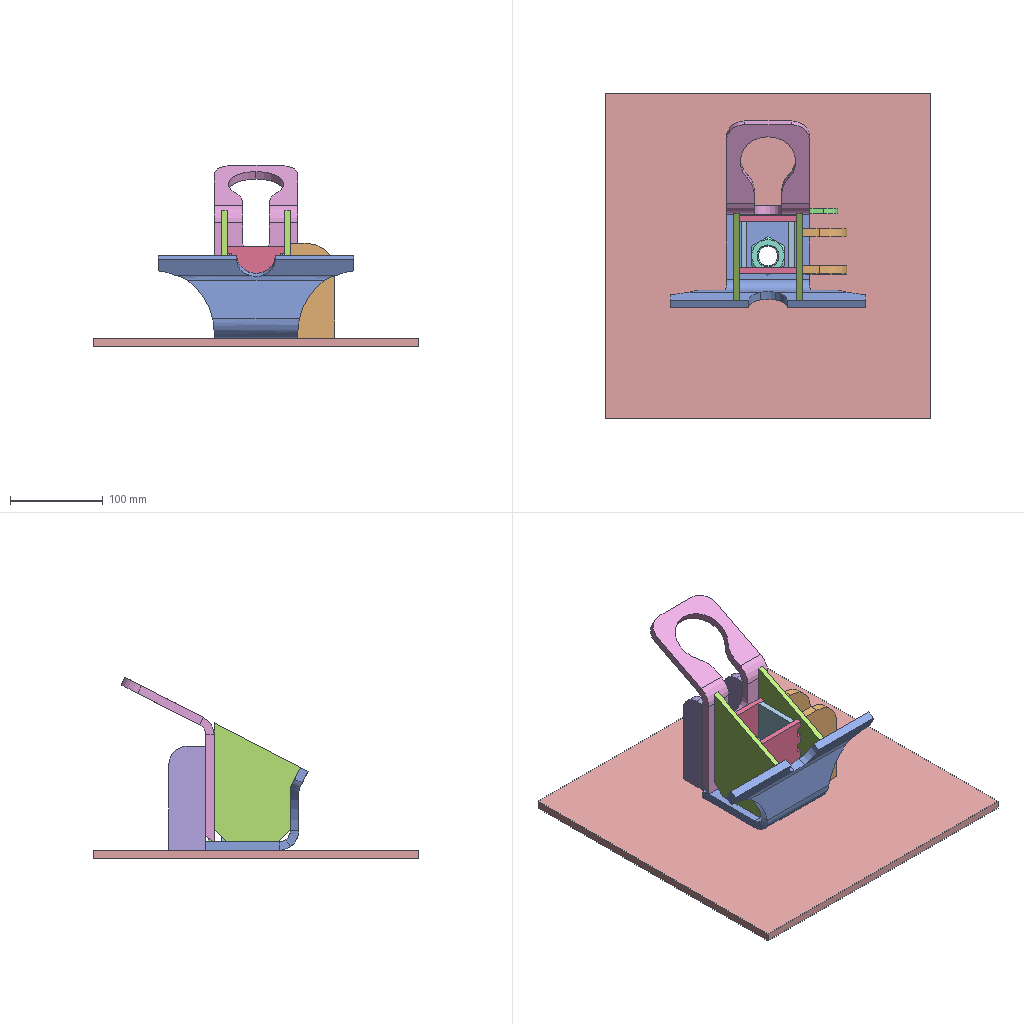Assembly | SolidWorks | 12 different items | 17 placed | box 350 x 350 x 195 mm
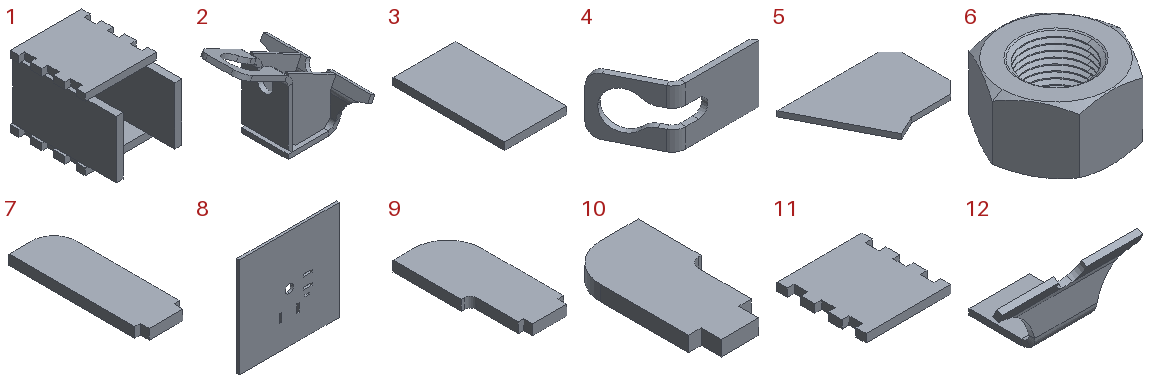Parts list (item | name | quantity | parent item | size | volume | features):
1 | (subassembly) | x1 | - | 62 x 90 x 62 mm | 98760 mm3 | -
2 | (subassembly) | x1 | - | 201.093 x 210 x 186 mm | 418946 mm3 | features CompositeCurve 1, MirrorCompFeat 1, ReferencePattern 1
3 | - | x2 | in 1 | 50 x 90 x 6 mm | 27000 mm3 | features FlatPattern 1, SMBaseFlange 1, SheetMetal 1
4 | - | x1 | in 2 | 177 x 100.092 x 90 mm | 136681 mm3 | features Fillet 2, Fold 2, ICE 2, UnFold 2, FlatPattern 1, SMBaseFlange 1, SheetMetal 1
5 | - | x2 | in 2 | 128 x 93 x 6 mm | 52464 mm3 | features FlatPattern 1, SMBaseFlange 1, SheetMetal 1
6 | - | x1 | in 2 | 41.569 x 36 x 21.5 mm | 15808 mm3 | features RevCut 2, Chamfer 1, Extrusion 1, LPattern 1
7 | - | x2 | - | 40 x 120 x 9 mm | 41707 mm3 | features FlatPattern 1, SMBaseFlange 1, SheetMetal 1
8 | - | x1 | - | 350 x 9 x 350 mm | 1086025 mm3 | features FlatPattern 1, ICE 1, SMBaseFlange 1, SheetMetal 1
9 | - | x2 | - | 48 x 110 x 9 mm | 41510 mm3 | features Fillet 1, FlatPattern 1, SMBaseFlange 1, SheetMetal 1
10 | - | x1 | - | 30 x 58 x 6 mm | 8701 mm3 | features FlatPattern 1, SMBaseFlange 1, SheetMetal 1
11 | - | x2 | in 1 | 62 x 65 x 6 mm | 22380 mm3 | features FlatPattern 1, SMBaseFlange 1, SheetMetal 1
12 | - | x1 | in 2 | 210 x 110.002 x 89.027 mm | 161533 mm3 | features SM3dBend 2, FlatPattern 1, SMBaseFlange 1, SheetMetal 1, UnFold 1
Mates (type | each side: item.copy, entity, surface, feature):
In the top assembly
Coincident | 8.1 face plane Base-Flange1 | 12.1 face plane Base-Flange1
Concentric | 8.1 face cylinder Base-Flange1 | 12.1 face cylinder Base-Flange1
Coincident | 8.1 face plane Base-Flange1 | 9.1 face plane Base-Flange1
Coincident | 8.1 face plane Cut-Extrude1 | 9.1 face plane Base-Flange1 | 2 times
Parallel | 8.1 face plane Base-Flange1 | 12.1 face plane Base-Flange1
Coincident | 8.1 face plane Base-Flange1 | 9.2 face plane Base-Flange1
Coincident | 8.1 face plane Cut-Extrude1 | 9.2 face plane Base-Flange1 | 2 times
Coincident | 8.1 face plane Cut-Extrude1 | 7.1 face plane Base-Flange1 | 2 times
Coincident | 8.1 face plane Base-Flange1 | 7.1 face plane Base-Flange1
Coincident | 8.1 face plane Base-Flange1 | 7.2 face plane Base-Flange1
Coincident | 8.1 face plane Cut-Extrude1 | 7.2 face plane Base-Flange1 | 2 times
Coincident | 8.1 face plane Cut-Extrude1 | 10.1 face plane Base-Flange1 | 2 times
Coincident | 8.1 face plane Base-Flange1 | 10.1 face plane Base-Flange1
Coincident | 12.1 face plane Base-Flange1 | 3.1 face plane Base-Flange1
Coincident | 5.1 face plane Base-Flange1 | 11.1 face plane Base-Flange1
DistanceDim | 11.1 face plane Base-Flange1 | 4.1 face plane Base-Flange1
In subassembly 1
Coincident | 11.2 face plane Base-Flange1 | 3.2 face plane Base-Flange1 | 2 times
Coincident | 11.2 face plane Base-Flange1 | 3.3 face plane Base-Flange1 | 2 times
Coincident | 3.2 face plane Base-Flange1 | 11.3 face plane Base-Flange1 | 2 times
DistanceDim | 3.2 face plane Base-Flange1 | 11.2 face plane Base-Flange1
DistanceDim | 11.2 face plane Base-Flange1 | 3.3 face plane Base-Flange1
In subassembly 2
Coincident | 12.2 face plane Base-Flange1 | 5.2 face plane Base-Flange1 | 2 times
DistanceDim | 5.2 face plane Base-Flange1 | 12.2 face plane Base-Flange1
Coincident | 12.2 face plane Base-Flange1 | 4.2 face plane Base-Flange1 | 3 times
Coincident | 12.2 face plane Base-Flange1 | 6.1 face plane BaseNut
Concentric | 12.2 face cylinder Base-Flange1 | 6.1 edge
Parallel | 12.2 face plane Base-Flange1 | 6.1 face plane BaseNut